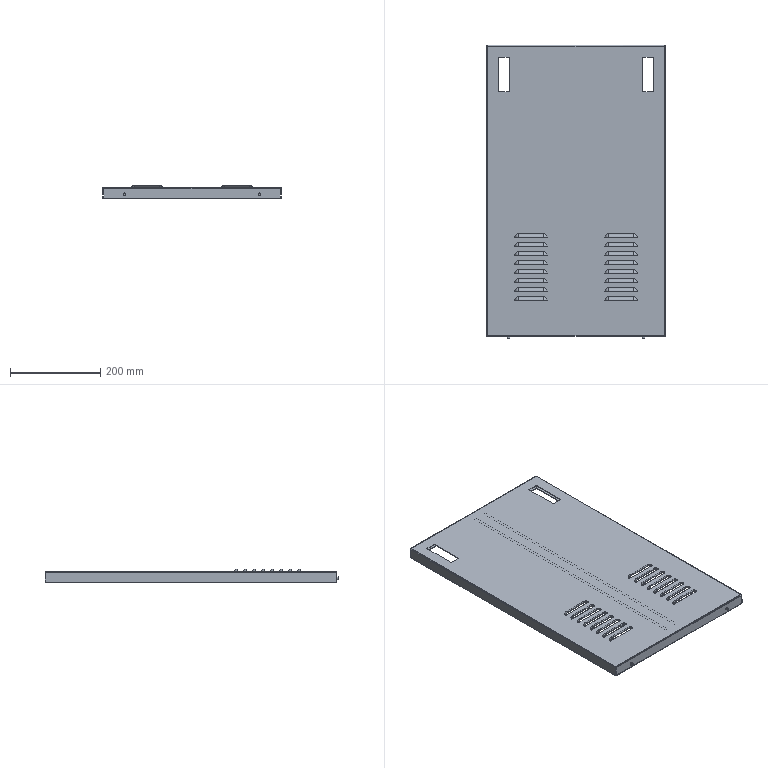Part | STEP file | FBDS-BJ-002 | 2 solids | 380 faces | box 396 x 651 x 31 mm | volume 529304 mm3 | plane 136 | cylinder 96 | torus 64 | sphere 64 | spline 16 | cone 4 | commonest cylinder face diameters 1 x16 4 x16 12 x16 15 x16 0.4 x12 3.4 x12